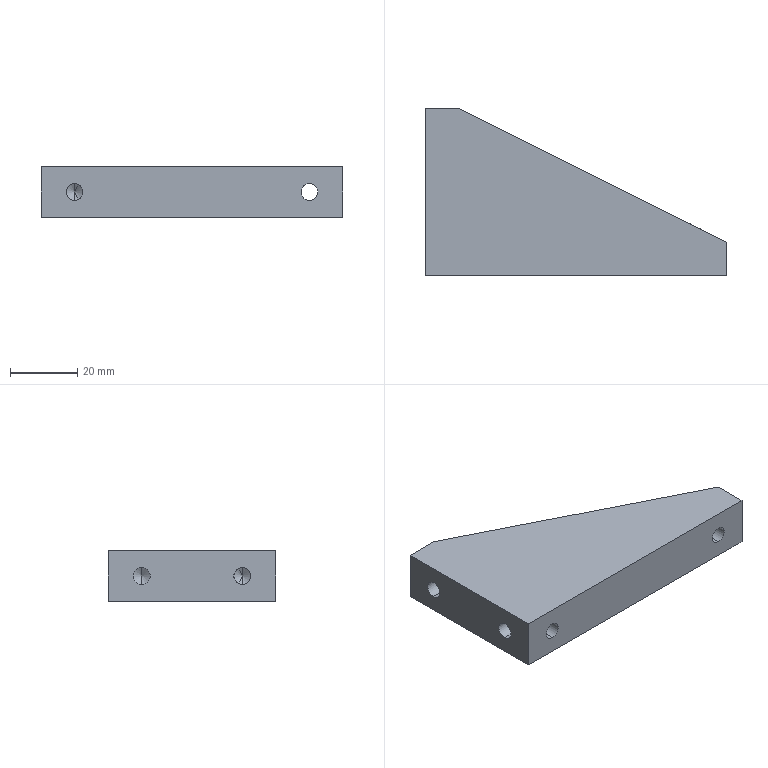Part | STEP file | 001-010-Waste reinforcing rib plate | 1 solid | 25 faces | box 90 x 50 x 15 mm | volume 42376 mm3 | cylinder 12 | plane 7 | cone 6 | commonest cylinder face diameters 5 x12